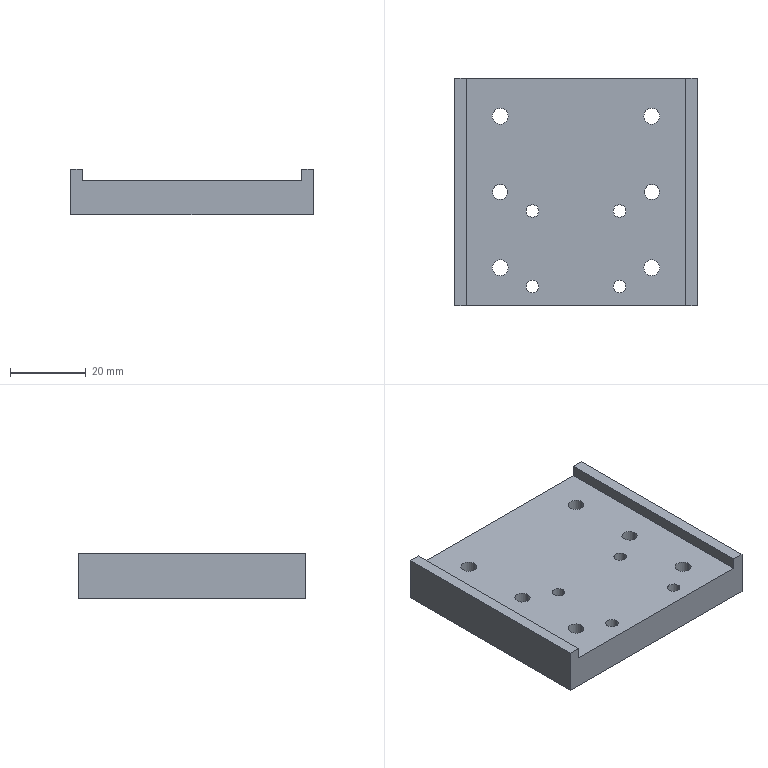Part | STEP file | 2065 Cylinder mounting plate 11 | 1 solid | 30 faces | box 64 x 60 x 12 mm | volume 34607 mm3 | cylinder 20 | plane 10 | commonest cylinder face diameters 3.3 x8 4.2 x8 4 x4